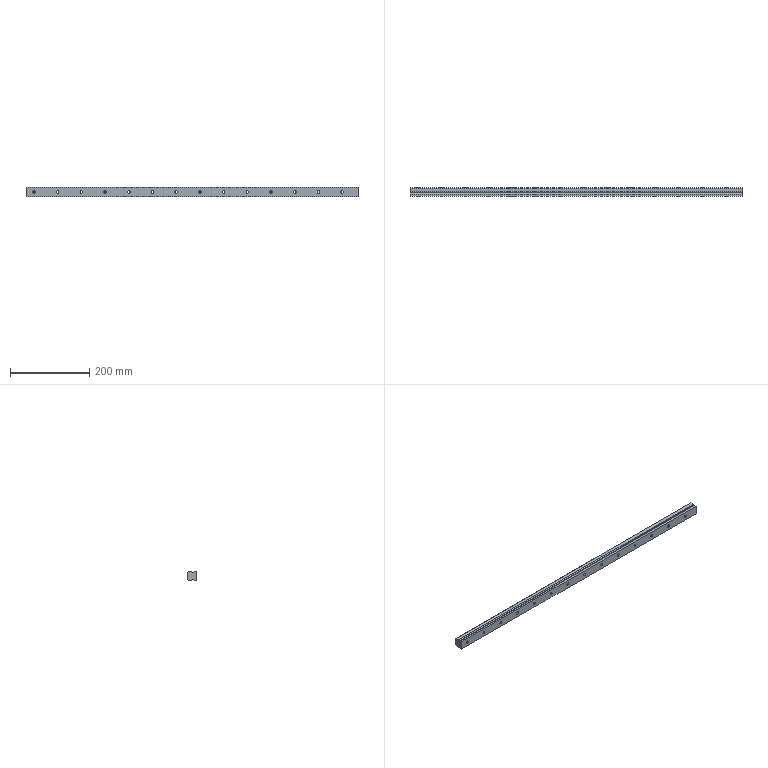Part | NX | features CBORE_HOLE 14, DATUM_CSYS 3, SKETCH 2, EXTRUDE 1, HOLE PACKAGE 1 | 1 solid | 58 faces | box 840 x 22 x 23 mm | volume 392391 mm3 | plane 30 | cylinder 28 | commonest cylinder face diameters 6.5 x14 11 x14
STEP:
#1=CARTESIAN_POINT('',(-420.,0.,-11.5));
#2=VERTEX_POINT('',#1);
#3=CARTESIAN_POINT('',(-420.,2.,-9.5));
#4=VERTEX_POINT('',#3);
#5=CARTESIAN_POINT('',(-420.,0.,-11.5));
#6=DIRECTION('',(0.,0.7071,0.7071));
#7=VECTOR('',#6,1000.);
#8=LINE('',#5,#7);
#9=EDGE_CURVE('',#2,#4,#8,.T.);
#10=ORIENTED_EDGE('',*,*,#9,.T.);
#11=CARTESIAN_POINT('',(420.,2.,-9.5));
#12=VERTEX_POINT('',#11);
#13=CARTESIAN_POINT('',(420.,2.,-9.5));
#14=DIRECTION('',(-1.,0.,0.));
#15=VECTOR('',#14,1000.);
#16=LINE('',#13,#15);
#17=EDGE_CURVE('',#12,#4,#16,.T.);
#18=ORIENTED_EDGE('',*,*,#17,.F.);
#19=CARTESIAN_POINT('',(420.,0.,-11.5));
#20=VERTEX_POINT('',#19);
#21=CARTESIAN_POINT('',(420.,0.,-11.5));
#22=DIRECTION('',(0.,0.7071,0.7071));
#23=VECTOR('',#22,1000.);
#24=LINE('',#21,#23);
#25=EDGE_CURVE('',#20,#12,#24,.T.);
#26=ORIENTED_EDGE('',*,*,#25,.F.);
#27=CARTESIAN_POINT('',(420.,0.,-11.5));
#28=DIRECTION('',(-1.,0.,0.));
#29=VECTOR('',#28,1000.);
#30=LINE('',#27,#29);
#31=EDGE_CURVE('',#20,#2,#30,.T.);
#32=ORIENTED_EDGE('',*,*,#31,.T.);
#33=EDGE_LOOP('',(#10,#18,#26,#32));
#34=FACE_BOUND('',#33,.T.);
#35=CARTESIAN_POINT('',(420.,0.,-11.5));
#36=DIRECTION('',(0.,-0.7071,0.7071));
#37=DIRECTION('',(0.,-0.7071,-0.7071));
#38=AXIS2_PLACEMENT_3D('',#35,#36,#37);
#39=PLANE('',#38);
#40=ADVANCED_FACE('',(#34),#39,.F.);
#41=CARTESIAN_POINT('',(-420.,4.,-9.5));
#42=VERTEX_POINT('',#41);
#43=CARTESIAN_POINT('',(-420.,2.,-9.5));
#44=DIRECTION('',(0.,1.,0.));
#45=VECTOR('',#44,1000.);
#46=LINE('',#43,#45);
#47=EDGE_CURVE('',#4,#42,#46,.T.);
#48=ORIENTED_EDGE('',*,*,#47,.T.);
#49=CARTESIAN_POINT('',(420.,4.,-9.5));
#50=VERTEX_POINT('',#49);
#51=CARTESIAN_POINT('',(420.,4.,-9.5));
#52=DIRECTION('',(-1.,0.,0.));
#53=VECTOR('',#52,1000.);
#54=LINE('',#51,#53);
#55=EDGE_CURVE('',#50,#42,#54,.T.);
#56=ORIENTED_EDGE('',*,*,#55,.F.);
#57=CARTESIAN_POINT('',(420.,2.,-9.5));
#58=DIRECTION('',(0.,1.,0.));
#59=VECTOR('',#58,1000.);
#60=LINE('',#57,#59);
#61=EDGE_CURVE('',#12,#50,#60,.T.);
#62=ORIENTED_EDGE('',*,*,#61,.F.);
#63=ORIENTED_EDGE('',*,*,#17,.T.);
#64=EDGE_LOOP('',(#48,#56,#62,#63));
#65=FACE_BOUND('',#64,.T.);
#66=CARTESIAN_POINT('',(420.,2.,-9.5));
#67=DIRECTION('',(0.,0.,1.));
#68=DIRECTION('',(1.,0.,0.));
#69=AXIS2_PLACEMENT_3D('',#66,#67,#68);
#70=PLANE('',#69);
#71=ADVANCED_FACE('',(#65),#70,.F.);
#72=CARTESIAN_POINT('',(-420.,6.,-11.5));
#73=VERTEX_POINT('',#72);
#74=CARTESIAN_POINT('',(-420.,4.,-9.5));
#75=DIRECTION('',(0.,0.7071,-0.7071));
#76=VECTOR('',#75,1000.);
#77=LINE('',#74,#76);
#78=EDGE_CURVE('',#42,#73,#77,.T.);
#79=ORIENTED_EDGE('',*,*,#78,.T.);
#80=CARTESIAN_POINT('',(420.,6.,-11.5));
#81=VERTEX_POINT('',#80);
#82=CARTESIAN_POINT('',(420.,6.,-11.5));
#83=DIRECTION('',(-1.,0.,0.));
#84=VECTOR('',#83,1000.);
#85=LINE('',#82,#84);
#86=EDGE_CURVE('',#81,#73,#85,.T.);
#87=ORIENTED_EDGE('',*,*,#86,.F.);
#88=CARTESIAN_POINT('',(420.,4.,-9.5));
#89=DIRECTION('',(0.,0.7071,-0.7071));
#90=VECTOR('',#89,1000.);
#91=LINE('',#88,#90);
#92=EDGE_CURVE('',#50,#81,#91,.T.);
#93=ORIENTED_EDGE('',*,*,#92,.F.);
#94=ORIENTED_EDGE('',*,*,#55,.T.);
#95=EDGE_LOOP('',(#79,#87,#93,#94));
#96=FACE_BOUND('',#95,.T.);
#97=CARTESIAN_POINT('',(420.,4.,-9.5));
#98=DIRECTION('',(0.,0.7071,0.7071));
#99=DIRECTION('',(0.,-0.7071,0.7071));
#100=AXIS2_PLACEMENT_3D('',#97,#98,#99);
#101=PLANE('',#100);
#102=ADVANCED_FACE('',(#96),#101,.F.);
#103=CARTESIAN_POINT('',(-420.,14.5,-11.5));
#104=VERTEX_POINT('',#103);
#105=CARTESIAN_POINT('',(-420.,6.,-11.5));
#106=DIRECTION('',(0.,1.,0.));
#107=VECTOR('',#106,1000.);
#108=LINE('',#105,#107);
#109=EDGE_CURVE('',#73,#104,#108,.T.);
#110=ORIENTED_EDGE('',*,*,#109,.T.);
#111=CARTESIAN_POINT('',(420.,14.5,-11.5));
#112=VERTEX_POINT('',#111);
#113=CARTESIAN_POINT('',(420.,14.5,-11.5));
#114=DIRECTION('',(-1.,0.,0.));
#115=VECTOR('',#114,1000.);
#116=LINE('',#113,#115);
#117=EDGE_CURVE('',#112,#104,#116,.T.);
#118=ORIENTED_EDGE('',*,*,#117,.F.);
#119=CARTESIAN_POINT('',(420.,6.,-11.5));
#120=DIRECTION('',(0.,1.,0.));
#121=VECTOR('',#120,1000.);
#122=LINE('',#119,#121);
#123=EDGE_CURVE('',#81,#112,#122,.T.);
#124=ORIENTED_EDGE('',*,*,#123,.F.);
#125=ORIENTED_EDGE('',*,*,#86,.T.);
#126=EDGE_LOOP('',(#110,#118,#124,#125));
#127=FACE_BOUND('',#126,.T.);
#128=CARTESIAN_POINT('',(420.,6.,-11.5));
#129=DIRECTION('',(0.,0.,1.));
#130=DIRECTION('',(0.,-1.,0.));
#131=AXIS2_PLACEMENT_3D('',#128,#129,#130);
#132=PLANE('',#131);
#133=ADVANCED_FACE('',(#127),#132,.F.);
#134=CARTESIAN_POINT('',(-420.,16.5,-9.5));
#135=VERTEX_POINT('',#134);
#136=CARTESIAN_POINT('',(-420.,14.5,-11.5));
#137=DIRECTION('',(0.,0.7071,0.7071));
#138=VECTOR('',#137,1000.);
#139=LINE('',#136,#138);
#140=EDGE_CURVE('',#104,#135,#139,.T.);
#141=ORIENTED_EDGE('',*,*,#140,.T.);
#142=CARTESIAN_POINT('',(420.,16.5,-9.5));
#143=VERTEX_POINT('',#142);
#144=CARTESIAN_POINT('',(420.,16.5,-9.5));
#145=DIRECTION('',(-1.,0.,0.));
#146=VECTOR('',#145,1000.);
#147=LINE('',#144,#146);
#148=EDGE_CURVE('',#143,#135,#147,.T.);
#149=ORIENTED_EDGE('',*,*,#148,.F.);
#150=CARTESIAN_POINT('',(420.,14.5,-11.5));
#151=DIRECTION('',(0.,0.7071,0.7071));
#152=VECTOR('',#151,1000.);
#153=LINE('',#150,#152);
#154=EDGE_CURVE('',#112,#143,#153,.T.);
#155=ORIENTED_EDGE('',*,*,#154,.F.);
#156=ORIENTED_EDGE('',*,*,#117,.T.);
#157=EDGE_LOOP('',(#141,#149,#155,#156));
#158=FACE_BOUND('',#157,.T.);
#159=CARTESIAN_POINT('',(420.,14.5,-11.5));
#160=DIRECTION('',(0.,-0.7071,0.7071));
#161=DIRECTION('',(0.,-0.7071,-0.7071));
#162=AXIS2_PLACEMENT_3D('',#159,#160,#161);
#163=PLANE('',#162);
#164=ADVANCED_FACE('',(#158),#163,.F.);
#165=CARTESIAN_POINT('',(380.,16.5,-5.5));
#166=VERTEX_POINT('',#165);
#167=CARTESIAN_POINT('',(380.,16.5,0.));
#168=DIRECTION('',(0.,-1.,0.));
#169=DIRECTION('',(0.,0.,-1.));
#170=AXIS2_PLACEMENT_3D('',#167,#168,#169);
#171=CIRCLE('',#170,5.5);
#172=EDGE_CURVE('',#166,#166,#171,.T.);
#173=ORIENTED_EDGE('',*,*,#172,.T.);
#174=EDGE_LOOP('',(#173));
#175=FACE_BOUND('',#174,.T.);
#176=CARTESIAN_POINT('',(320.,16.5,-5.5));
#177=VERTEX_POINT('',#176);
#178=CARTESIAN_POINT('',(320.,16.5,0.));
#179=DIRECTION('',(0.,-1.,0.));
#180=DIRECTION('',(0.,0.,-1.));
#181=AXIS2_PLACEMENT_3D('',#178,#179,#180);
#182=CIRCLE('',#181,5.5);
#183=EDGE_CURVE('',#177,#177,#182,.T.);
#184=ORIENTED_EDGE('',*,*,#183,.T.);
#185=EDGE_LOOP('',(#184));
#186=FACE_BOUND('',#185,.T.);
#187=CARTESIAN_POINT('',(260.,16.5,-5.5));
#188=VERTEX_POINT('',#187);
#189=CARTESIAN_POINT('',(260.,16.5,0.));
#190=DIRECTION('',(0.,-1.,0.));
#191=DIRECTION('',(0.,0.,-1.));
#192=AXIS2_PLACEMENT_3D('',#189,#190,#191);
#193=CIRCLE('',#192,5.5);
#194=EDGE_CURVE('',#188,#188,#193,.T.);
#195=ORIENTED_EDGE('',*,*,#194,.T.);
#196=EDGE_LOOP('',(#195));
#197=FACE_BOUND('',#196,.T.);
#198=CARTESIAN_POINT('',(200.,16.5,-5.5));
#199=VERTEX_POINT('',#198);
#200=CARTESIAN_POINT('',(200.,16.5,0.));
#201=DIRECTION('',(0.,-1.,0.));
#202=DIRECTION('',(0.,0.,-1.));
#203=AXIS2_PLACEMENT_3D('',#200,#201,#202);
#204=CIRCLE('',#203,5.5);
#205=EDGE_CURVE('',#199,#199,#204,.T.);
#206=ORIENTED_EDGE('',*,*,#205,.T.);
#207=EDGE_LOOP('',(#206));
#208=FACE_BOUND('',#207,.T.);
#209=CARTESIAN_POINT('',(140.,16.5,-5.5));
#210=VERTEX_POINT('',#209);
#211=CARTESIAN_POINT('',(140.,16.5,0.));
#212=DIRECTION('',(0.,-1.,0.));
#213=DIRECTION('',(0.,0.,-1.));
#214=AXIS2_PLACEMENT_3D('',#211,#212,#213);
#215=CIRCLE('',#214,5.5);
#216=EDGE_CURVE('',#210,#210,#215,.T.);
#217=ORIENTED_EDGE('',*,*,#216,.T.);
#218=EDGE_LOOP('',(#217));
#219=FACE_BOUND('',#218,.T.);
#220=CARTESIAN_POINT('',(80.,16.5,-5.5));
#221=VERTEX_POINT('',#220);
#222=CARTESIAN_POINT('',(80.,16.5,0.));
#223=DIRECTION('',(0.,-1.,0.));
#224=DIRECTION('',(0.,0.,-1.));
#225=AXIS2_PLACEMENT_3D('',#222,#223,#224);
#226=CIRCLE('',#225,5.5);
#227=EDGE_CURVE('',#221,#221,#226,.T.);
#228=ORIENTED_EDGE('',*,*,#227,.T.);
#229=EDGE_LOOP('',(#228));
#230=FACE_BOUND('',#229,.T.);
#231=CARTESIAN_POINT('',(20.,16.5,-5.5));
#232=VERTEX_POINT('',#231);
#233=CARTESIAN_POINT('',(20.,16.5,0.));
#234=DIRECTION('',(0.,-1.,0.));
#235=DIRECTION('',(0.,0.,-1.));
#236=AXIS2_PLACEMENT_3D('',#233,#234,#235);
#237=CIRCLE('',#236,5.5);
#238=EDGE_CURVE('',#232,#232,#237,.T.);
#239=ORIENTED_EDGE('',*,*,#238,.T.);
#240=EDGE_LOOP('',(#239));
#241=FACE_BOUND('',#240,.T.);
#242=CARTESIAN_POINT('',(-40.,16.5,-5.5));
#243=VERTEX_POINT('',#242);
#244=CARTESIAN_POINT('',(-40.,16.5,0.));
#245=DIRECTION('',(0.,-1.,0.));
#246=DIRECTION('',(0.,0.,-1.));
#247=AXIS2_PLACEMENT_3D('',#244,#245,#246);
#248=CIRCLE('',#247,5.5);
#249=EDGE_CURVE('',#243,#243,#248,.T.);
#250=ORIENTED_EDGE('',*,*,#249,.T.);
#251=EDGE_LOOP('',(#250));
#252=FACE_BOUND('',#251,.T.);
#253=CARTESIAN_POINT('',(-100.,16.5,-5.5));
#254=VERTEX_POINT('',#253);
#255=CARTESIAN_POINT('',(-100.,16.5,0.));
#256=DIRECTION('',(0.,-1.,0.));
#257=DIRECTION('',(0.,0.,-1.));
#258=AXIS2_PLACEMENT_3D('',#255,#256,#257);
#259=CIRCLE('',#258,5.5);
#260=EDGE_CURVE('',#254,#254,#259,.T.);
#261=ORIENTED_EDGE('',*,*,#260,.T.);
#262=EDGE_LOOP('',(#261));
#263=FACE_BOUND('',#262,.T.);
#264=CARTESIAN_POINT('',(-160.,16.5,-5.5));
#265=VERTEX_POINT('',#264);
#266=CARTESIAN_POINT('',(-160.,16.5,0.));
#267=DIRECTION('',(0.,-1.,0.));
#268=DIRECTION('',(0.,0.,-1.));
#269=AXIS2_PLACEMENT_3D('',#266,#267,#268);
#270=CIRCLE('',#269,5.5);
#271=EDGE_CURVE('',#265,#265,#270,.T.);
#272=ORIENTED_EDGE('',*,*,#271,.T.);
#273=EDGE_LOOP('',(#272));
#274=FACE_BOUND('',#273,.T.);
#275=CARTESIAN_POINT('',(-220.,16.5,-5.5));
#276=VERTEX_POINT('',#275);
#277=CARTESIAN_POINT('',(-220.,16.5,0.));
#278=DIRECTION('',(0.,-1.,0.));
#279=DIRECTION('',(0.,0.,-1.));
#280=AXIS2_PLACEMENT_3D('',#277,#278,#279);
#281=CIRCLE('',#280,5.5);
#282=EDGE_CURVE('',#276,#276,#281,.T.);
#283=ORIENTED_EDGE('',*,*,#282,.T.);
#284=EDGE_LOOP('',(#283));
#285=FACE_BOUND('',#284,.T.);
#286=CARTESIAN_POINT('',(-280.,16.5,-5.5));
#287=VERTEX_POINT('',#286);
#288=CARTESIAN_POINT('',(-280.,16.5,0.));
#289=DIRECTION('',(0.,-1.,0.));
#290=DIRECTION('',(0.,0.,-1.));
#291=AXIS2_PLACEMENT_3D('',#288,#289,#290);
#292=CIRCLE('',#291,5.5);
#293=EDGE_CURVE('',#287,#287,#292,.T.);
#294=ORIENTED_EDGE('',*,*,#293,.T.);
#295=EDGE_LOOP('',(#294));
#296=FACE_BOUND('',#295,.T.);
#297=CARTESIAN_POINT('',(-340.,16.5,-5.5));
#298=VERTEX_POINT('',#297);
#299=CARTESIAN_POINT('',(-340.,16.5,0.));
#300=DIRECTION('',(0.,-1.,0.));
#301=DIRECTION('',(0.,0.,-1.));
#302=AXIS2_PLACEMENT_3D('',#299,#300,#301);
#303=CIRCLE('',#302,5.5);
#304=EDGE_CURVE('',#298,#298,#303,.T.);
#305=ORIENTED_EDGE('',*,*,#304,.T.);
#306=EDGE_LOOP('',(#305));
#307=FACE_BOUND('',#306,.T.);
#308=CARTESIAN_POINT('',(-400.,16.5,-5.5));
#309=VERTEX_POINT('',#308);
#310=CARTESIAN_POINT('',(-400.,16.5,0.));
#311=DIRECTION('',(0.,-1.,0.));
#312=DIRECTION('',(0.,0.,-1.));
#313=AXIS2_PLACEMENT_3D('',#310,#311,#312);
#314=CIRCLE('',#313,5.5);
#315=EDGE_CURVE('',#309,#309,#314,.T.);
#316=ORIENTED_EDGE('',*,*,#315,.T.);
#317=EDGE_LOOP('',(#316));
#318=FACE_BOUND('',#317,.T.);
#319=CARTESIAN_POINT('',(-420.,16.5,9.5));
#320=VERTEX_POINT('',#319);
#321=CARTESIAN_POINT('',(-420.,16.5,0.));
#322=DIRECTION('',(0.,0.,1.));
#323=VECTOR('',#322,1000.);
#324=LINE('',#321,#323);
#325=EDGE_CURVE('',#135,#320,#324,.T.);
#326=ORIENTED_EDGE('',*,*,#325,.T.);
#327=CARTESIAN_POINT('',(420.,16.5,9.5));
#328=VERTEX_POINT('',#327);
#329=CARTESIAN_POINT('',(420.,16.5,9.5));
#330=DIRECTION('',(-1.,0.,0.));
#331=VECTOR('',#330,1000.);
#332=LINE('',#329,#331);
#333=EDGE_CURVE('',#328,#320,#332,.T.);
#334=ORIENTED_EDGE('',*,*,#333,.F.);
#335=CARTESIAN_POINT('',(420.,16.5,-9.5));
#336=DIRECTION('',(0.,0.,1.));
#337=VECTOR('',#336,1000.);
#338=LINE('',#335,#337);
#339=EDGE_CURVE('',#143,#328,#338,.T.);
#340=ORIENTED_EDGE('',*,*,#339,.F.);
#341=ORIENTED_EDGE('',*,*,#148,.T.);
#342=EDGE_LOOP('',(#326,#334,#340,#341));
#343=FACE_BOUND('',#342,.T.);
#344=CARTESIAN_POINT('',(420.,16.5,0.));
#345=DIRECTION('',(0.,-1.,0.));
#346=DIRECTION('',(0.,0.,-1.));
#347=AXIS2_PLACEMENT_3D('',#344,#345,#346);
#348=PLANE('',#347);
#349=ADVANCED_FACE('',(#175,#186,#197,#208,#219,#230,#241,#252,#263,#274,#285,#296,#307,#318,#343),#348,.F.);
#350=CARTESIAN_POINT('',(-420.,14.5,11.5));
#351=VERTEX_POINT('',#350);
#352=CARTESIAN_POINT('',(-420.,16.5,9.5));
#353=DIRECTION('',(0.,-0.7071,0.7071));
#354=VECTOR('',#353,1000.);
#355=LINE('',#352,#354);
#356=EDGE_CURVE('',#320,#351,#355,.T.);
#357=ORIENTED_EDGE('',*,*,#356,.T.);
#358=CARTESIAN_POINT('',(420.,14.5,11.5));
#359=VERTEX_POINT('',#358);
#360=CARTESIAN_POINT('',(420.,14.5,11.5));
#361=DIRECTION('',(-1.,0.,0.));
#362=VECTOR('',#361,1000.);
#363=LINE('',#360,#362);
#364=EDGE_CURVE('',#359,#351,#363,.T.);
#365=ORIENTED_EDGE('',*,*,#364,.F.);
#366=CARTESIAN_POINT('',(420.,16.5,9.5));
#367=DIRECTION('',(0.,-0.7071,0.7071));
#368=VECTOR('',#367,1000.);
#369=LINE('',#366,#368);
#370=EDGE_CURVE('',#328,#359,#369,.T.);
#371=ORIENTED_EDGE('',*,*,#370,.F.);
#372=ORIENTED_EDGE('',*,*,#333,.T.);
#373=EDGE_LOOP('',(#357,#365,#371,#372));
#374=FACE_BOUND('',#373,.T.);
#375=CARTESIAN_POINT('',(420.,16.5,9.5));
#376=DIRECTION('',(0.,-0.7071,-0.7071));
#377=DIRECTION('',(0.,0.7071,-0.7071));
#378=AXIS2_PLACEMENT_3D('',#375,#376,#377);
#379=PLANE('',#378);
#380=ADVANCED_FACE('',(#374),#379,.F.);
#381=CARTESIAN_POINT('',(-420.,6.,11.5));
#382=VERTEX_POINT('',#381);
#383=CARTESIAN_POINT('',(-420.,14.5,11.5));
#384=DIRECTION('',(0.,-1.,0.));
#385=VECTOR('',#384,1000.);
#386=LINE('',#383,#385);
#387=EDGE_CURVE('',#351,#382,#386,.T.);
#388=ORIENTED_EDGE('',*,*,#387,.T.);
#389=CARTESIAN_POINT('',(420.,6.,11.5));
#390=VERTEX_POINT('',#389);
#391=CARTESIAN_POINT('',(420.,6.,11.5));
#392=DIRECTION('',(-1.,0.,0.));
#393=VECTOR('',#392,1000.);
#394=LINE('',#391,#393);
#395=EDGE_CURVE('',#390,#382,#394,.T.);
#396=ORIENTED_EDGE('',*,*,#395,.F.);
#397=CARTESIAN_POINT('',(420.,14.5,11.5));
#398=DIRECTION('',(0.,-1.,0.));
#399=VECTOR('',#398,1000.);
#400=LINE('',#397,#399);
#401=EDGE_CURVE('',#359,#390,#400,.T.);
#402=ORIENTED_EDGE('',*,*,#401,.F.);
#403=ORIENTED_EDGE('',*,*,#364,.T.);
#404=EDGE_LOOP('',(#388,#396,#402,#403));
#405=FACE_BOUND('',#404,.T.);
#406=CARTESIAN_POINT('',(420.,14.5,11.5));
#407=DIRECTION('',(0.,0.,-1.));
#408=DIRECTION('',(0.,1.,0.));
#409=AXIS2_PLACEMENT_3D('',#406,#407,#408);
#410=PLANE('',#409);
#411=ADVANCED_FACE('',(#405),#410,.F.);
#412=CARTESIAN_POINT('',(-420.,4.,9.5));
#413=VERTEX_POINT('',#412);
#414=CARTESIAN_POINT('',(-420.,6.,11.5));
#415=DIRECTION('',(0.,-0.7071,-0.7071));
#416=VECTOR('',#415,1000.);
#417=LINE('',#414,#416);
#418=EDGE_CURVE('',#382,#413,#417,.T.);
#419=ORIENTED_EDGE('',*,*,#418,.T.);
#420=CARTESIAN_POINT('',(420.,4.,9.5));
#421=VERTEX_POINT('',#420);
#422=CARTESIAN_POINT('',(420.,4.,9.5));
#423=DIRECTION('',(-1.,0.,0.));
#424=VECTOR('',#423,1000.);
#425=LINE('',#422,#424);
#426=EDGE_CURVE('',#421,#413,#425,.T.);
#427=ORIENTED_EDGE('',*,*,#426,.F.);
#428=CARTESIAN_POINT('',(420.,6.,11.5));
#429=DIRECTION('',(0.,-0.7071,-0.7071));
#430=VECTOR('',#429,1000.);
#431=LINE('',#428,#430);
#432=EDGE_CURVE('',#390,#421,#431,.T.);
#433=ORIENTED_EDGE('',*,*,#432,.F.);
#434=ORIENTED_EDGE('',*,*,#395,.T.);
#435=EDGE_LOOP('',(#419,#427,#433,#434));
#436=FACE_BOUND('',#435,.T.);
#437=CARTESIAN_POINT('',(420.,6.,11.5));
#438=DIRECTION('',(0.,0.7071,-0.7071));
#439=DIRECTION('',(0.,0.7071,0.7071));
#440=AXIS2_PLACEMENT_3D('',#437,#438,#439);
#441=PLANE('',#440);
#442=ADVANCED_FACE('',(#436),#441,.F.);
#443=CARTESIAN_POINT('',(-420.,2.,9.5));
#444=VERTEX_POINT('',#443);
#445=CARTESIAN_POINT('',(-420.,4.,9.5));
#446=DIRECTION('',(0.,-1.,0.));
#447=VECTOR('',#446,1000.);
#448=LINE('',#445,#447);
#449=EDGE_CURVE('',#413,#444,#448,.T.);
#450=ORIENTED_EDGE('',*,*,#449,.T.);
#451=CARTESIAN_POINT('',(420.,2.,9.5));
#452=VERTEX_POINT('',#451);
#453=CARTESIAN_POINT('',(420.,2.,9.5));
#454=DIRECTION('',(-1.,0.,0.));
#455=VECTOR('',#454,1000.);
#456=LINE('',#453,#455);
#457=EDGE_CURVE('',#452,#444,#456,.T.);
#458=ORIENTED_EDGE('',*,*,#457,.F.);
#459=CARTESIAN_POINT('',(420.,4.,9.5));
#460=DIRECTION('',(0.,-1.,0.));
#461=VECTOR('',#460,1000.);
#462=LINE('',#459,#461);
#463=EDGE_CURVE('',#421,#452,#462,.T.);
#464=ORIENTED_EDGE('',*,*,#463,.F.);
#465=ORIENTED_EDGE('',*,*,#426,.T.);
#466=EDGE_LOOP('',(#450,#458,#464,#465));
#467=FACE_BOUND('',#466,.T.);
#468=CARTESIAN_POINT('',(420.,4.,9.5));
#469=DIRECTION('',(0.,0.,-1.));
#470=DIRECTION('',(-1.,0.,0.));
#471=AXIS2_PLACEMENT_3D('',#468,#469,#470);
#472=PLANE('',#471);
#473=ADVANCED_FACE('',(#467),#472,.F.);
#474=CARTESIAN_POINT('',(-420.,0.,11.5));
#475=VERTEX_POINT('',#474);
#476=CARTESIAN_POINT('',(-420.,2.,9.5));
#477=DIRECTION('',(0.,-0.7071,0.7071));
#478=VECTOR('',#477,1000.);
#479=LINE('',#476,#478);
#480=EDGE_CURVE('',#444,#475,#479,.T.);
#481=ORIENTED_EDGE('',*,*,#480,.T.);
#482=CARTESIAN_POINT('',(420.,0.,11.5));
#483=VERTEX_POINT('',#482);
#484=CARTESIAN_POINT('',(420.,0.,11.5));
#485=DIRECTION('',(-1.,0.,0.));
#486=VECTOR('',#485,1000.);
#487=LINE('',#484,#486);
#488=EDGE_CURVE('',#483,#475,#487,.T.);
#489=ORIENTED_EDGE('',*,*,#488,.F.);
#490=CARTESIAN_POINT('',(420.,2.,9.5));
#491=DIRECTION('',(0.,-0.7071,0.7071));
#492=VECTOR('',#491,1000.);
#493=LINE('',#490,#492);
#494=EDGE_CURVE('',#452,#483,#493,.T.);
#495=ORIENTED_EDGE('',*,*,#494,.F.);
#496=ORIENTED_EDGE('',*,*,#457,.T.);
#497=EDGE_LOOP('',(#481,#489,#495,#496));
#498=FACE_BOUND('',#497,.T.);
#499=CARTESIAN_POINT('',(420.,2.,9.5));
#500=DIRECTION('',(0.,-0.7071,-0.7071));
#501=DIRECTION('',(0.,0.7071,-0.7071));
#502=AXIS2_PLACEMENT_3D('',#499,#500,#501);
#503=PLANE('',#502);
#504=ADVANCED_FACE('',(#498),#503,.F.);
#505=CARTESIAN_POINT('',(-420.,-5.5,11.5));
#506=VERTEX_POINT('',#505);
#507=CARTESIAN_POINT('',(-420.,0.,11.5));
#508=DIRECTION('',(0.,-1.,0.));
#509=VECTOR('',#508,1000.);
#510=LINE('',#507,#509);
#511=EDGE_CURVE('',#475,#506,#510,.T.);
#512=ORIENTED_EDGE('',*,*,#511,.T.);
#513=CARTESIAN_POINT('',(420.,-5.5,11.5));
#514=VERTEX_POINT('',#513);
#515=CARTESIAN_POINT('',(420.,-5.5,11.5));
#516=DIRECTION('',(-1.,0.,0.));
#517=VECTOR('',#516,1000.);
#518=LINE('',#515,#517);
#519=EDGE_CURVE('',#514,#506,#518,.T.);
#520=ORIENTED_EDGE('',*,*,#519,.F.);
#521=CARTESIAN_POINT('',(420.,0.,11.5));
#522=DIRECTION('',(0.,-1.,0.));
#523=VECTOR('',#522,1000.);
#524=LINE('',#521,#523);
#525=EDGE_CURVE('',#483,#514,#524,.T.);
#526=ORIENTED_EDGE('',*,*,#525,.F.);
#527=ORIENTED_EDGE('',*,*,#488,.T.);
#528=EDGE_LOOP('',(#512,#520,#526,#527));
#529=FACE_BOUND('',#528,.T.);
#530=CARTESIAN_POINT('',(420.,0.,11.5));
#531=DIRECTION('',(0.,0.,-1.));
#532=DIRECTION('',(0.,1.,0.));
#533=AXIS2_PLACEMENT_3D('',#530,#531,#532);
#534=PLANE('',#533);
#535=ADVANCED_FACE('',(#529),#534,.F.);
#536=CARTESIAN_POINT('',(380.,-5.5,3.25));
#537=VERTEX_POINT('',#536);
#538=CARTESIAN_POINT('',(380.,-5.5,0.));
#539=DIRECTION('',(0.,1.,0.));
#540=DIRECTION('',(0.,0.,1.));
#541=AXIS2_PLACEMENT_3D('',#538,#539,#540);
#542=CIRCLE('',#541,3.25);
#543=EDGE_CURVE('',#537,#537,#542,.T.);
#544=ORIENTED_EDGE('',*,*,#543,.T.);
#545=EDGE_LOOP('',(#544));
#546=FACE_BOUND('',#545,.T.);
#547=CARTESIAN_POINT('',(320.,-5.5,3.25));
#548=VERTEX_POINT('',#547);
#549=CARTESIAN_POINT('',(320.,-5.5,0.));
#550=DIRECTION('',(0.,1.,0.));
#551=DIRECTION('',(0.,0.,1.));
#552=AXIS2_PLACEMENT_3D('',#549,#550,#551);
#553=CIRCLE('',#552,3.25);
#554=EDGE_CURVE('',#548,#548,#553,.T.);
#555=ORIENTED_EDGE('',*,*,#554,.T.);
#556=EDGE_LOOP('',(#555));
#557=FACE_BOUND('',#556,.T.);
#558=CARTESIAN_POINT('',(260.,-5.5,3.25));
#559=VERTEX_POINT('',#558);
#560=CARTESIAN_POINT('',(260.,-5.5,0.));
#561=DIRECTION('',(0.,1.,0.));
#562=DIRECTION('',(0.,0.,1.));
#563=AXIS2_PLACEMENT_3D('',#560,#561,#562);
#564=CIRCLE('',#563,3.25);
#565=EDGE_CURVE('',#559,#559,#564,.T.);
#566=ORIENTED_EDGE('',*,*,#565,.T.);
#567=EDGE_LOOP('',(#566));
#568=FACE_BOUND('',#567,.T.);
#569=CARTESIAN_POINT('',(200.,-5.5,3.25));
#570=VERTEX_POINT('',#569);
#571=CARTESIAN_POINT('',(200.,-5.5,0.));
#572=DIRECTION('',(0.,1.,0.));
#573=DIRECTION('',(0.,0.,1.));
#574=AXIS2_PLACEMENT_3D('',#571,#572,#573);
#575=CIRCLE('',#574,3.25);
#576=EDGE_CURVE('',#570,#570,#575,.T.);
#577=ORIENTED_EDGE('',*,*,#576,.T.);
#578=EDGE_LOOP('',(#577));
#579=FACE_BOUND('',#578,.T.);
#580=CARTESIAN_POINT('',(140.,-5.5,3.25));
#581=VERTEX_POINT('',#580);
#582=CARTESIAN_POINT('',(140.,-5.5,0.));
#583=DIRECTION('',(0.,1.,0.));
#584=DIRECTION('',(0.,0.,1.));
#585=AXIS2_PLACEMENT_3D('',#582,#583,#584);
#586=CIRCLE('',#585,3.25);
#587=EDGE_CURVE('',#581,#581,#586,.T.);
#588=ORIENTED_EDGE('',*,*,#587,.T.);
#589=EDGE_LOOP('',(#588));
#590=FACE_BOUND('',#589,.T.);
#591=CARTESIAN_POINT('',(80.,-5.5,3.25));
#592=VERTEX_POINT('',#591);
#593=CARTESIAN_POINT('',(80.,-5.5,0.));
#594=DIRECTION('',(0.,1.,0.));
#595=DIRECTION('',(0.,0.,1.));
#596=AXIS2_PLACEMENT_3D('',#593,#594,#595);
#597=CIRCLE('',#596,3.25);
#598=EDGE_CURVE('',#592,#592,#597,.T.);
#599=ORIENTED_EDGE('',*,*,#598,.T.);
#600=EDGE_LOOP('',(#599));
#601=FACE_BOUND('',#600,.T.);
#602=CARTESIAN_POINT('',(20.,-5.5,3.25));
#603=VERTEX_POINT('',#602);
#604=CARTESIAN_POINT('',(20.,-5.5,0.));
#605=DIRECTION('',(0.,1.,0.));
#606=DIRECTION('',(0.,0.,1.));
#607=AXIS2_PLACEMENT_3D('',#604,#605,#606);
#608=CIRCLE('',#607,3.25);
#609=EDGE_CURVE('',#603,#603,#608,.T.);
#610=ORIENTED_EDGE('',*,*,#609,.T.);
#611=EDGE_LOOP('',(#610));
#612=FACE_BOUND('',#611,.T.);
#613=CARTESIAN_POINT('',(-40.,-5.5,3.25));
#614=VERTEX_POINT('',#613);
#615=CARTESIAN_POINT('',(-40.,-5.5,0.));
#616=DIRECTION('',(0.,1.,0.));
#617=DIRECTION('',(0.,0.,1.));
#618=AXIS2_PLACEMENT_3D('',#615,#616,#617);
#619=CIRCLE('',#618,3.25);
#620=EDGE_CURVE('',#614,#614,#619,.T.);
#621=ORIENTED_EDGE('',*,*,#620,.T.);
#622=EDGE_LOOP('',(#621));
#623=FACE_BOUND('',#622,.T.);
#624=CARTESIAN_POINT('',(-100.,-5.5,3.25));
#625=VERTEX_POINT('',#624);
#626=CARTESIAN_POINT('',(-100.,-5.5,0.));
#627=DIRECTION('',(0.,1.,0.));
#628=DIRECTION('',(0.,0.,1.));
#629=AXIS2_PLACEMENT_3D('',#626,#627,#628);
#630=CIRCLE('',#629,3.25);
#631=EDGE_CURVE('',#625,#625,#630,.T.);
#632=ORIENTED_EDGE('',*,*,#631,.T.);
#633=EDGE_LOOP('',(#632));
#634=FACE_BOUND('',#633,.T.);
#635=CARTESIAN_POINT('',(-160.,-5.5,3.25));
#636=VERTEX_POINT('',#635);
#637=CARTESIAN_POINT('',(-160.,-5.5,0.));
#638=DIRECTION('',(0.,1.,0.));
#639=DIRECTION('',(0.,0.,1.));
#640=AXIS2_PLACEMENT_3D('',#637,#638,#639);
#641=CIRCLE('',#640,3.25);
#642=EDGE_CURVE('',#636,#636,#641,.T.);
#643=ORIENTED_EDGE('',*,*,#642,.T.);
#644=EDGE_LOOP('',(#643));
#645=FACE_BOUND('',#644,.T.);
#646=CARTESIAN_POINT('',(-220.,-5.5,3.25));
#647=VERTEX_POINT('',#646);
#648=CARTESIAN_POINT('',(-220.,-5.5,0.));
#649=DIRECTION('',(0.,1.,0.));
#650=DIRECTION('',(0.,0.,1.));
#651=AXIS2_PLACEMENT_3D('',#648,#649,#650);
#652=CIRCLE('',#651,3.25);
#653=EDGE_CURVE('',#647,#647,#652,.T.);
#654=ORIENTED_EDGE('',*,*,#653,.T.);
#655=EDGE_LOOP('',(#654));
#656=FACE_BOUND('',#655,.T.);
#657=CARTESIAN_POINT('',(-280.,-5.5,3.25));
#658=VERTEX_POINT('',#657);
#659=CARTESIAN_POINT('',(-280.,-5.5,0.));
#660=DIRECTION('',(0.,1.,0.));
#661=DIRECTION('',(0.,0.,1.));
#662=AXIS2_PLACEMENT_3D('',#659,#660,#661);
#663=CIRCLE('',#662,3.25);
#664=EDGE_CURVE('',#658,#658,#663,.T.);
#665=ORIENTED_EDGE('',*,*,#664,.T.);
#666=EDGE_LOOP('',(#665));
#667=FACE_BOUND('',#666,.T.);
#668=CARTESIAN_POINT('',(-340.,-5.5,3.25));
#669=VERTEX_POINT('',#668);
#670=CARTESIAN_POINT('',(-340.,-5.5,0.));
#671=DIRECTION('',(0.,1.,0.));
#672=DIRECTION('',(0.,0.,1.));
#673=AXIS2_PLACEMENT_3D('',#670,#671,#672);
#674=CIRCLE('',#673,3.25);
#675=EDGE_CURVE('',#669,#669,#674,.T.);
#676=ORIENTED_EDGE('',*,*,#675,.T.);
#677=EDGE_LOOP('',(#676));
#678=FACE_BOUND('',#677,.T.);
#679=CARTESIAN_POINT('',(-400.,-5.5,3.25));
#680=VERTEX_POINT('',#679);
#681=CARTESIAN_POINT('',(-400.,-5.5,0.));
#682=DIRECTION('',(0.,1.,0.));
#683=DIRECTION('',(0.,0.,1.));
#684=AXIS2_PLACEMENT_3D('',#681,#682,#683);
#685=CIRCLE('',#684,3.25);
#686=EDGE_CURVE('',#680,#680,#685,.T.);
#687=ORIENTED_EDGE('',*,*,#686,.T.);
#688=EDGE_LOOP('',(#687));
#689=FACE_BOUND('',#688,.T.);
#690=CARTESIAN_POINT('',(-420.,-5.5,-11.5));
#691=VERTEX_POINT('',#690);
#692=CARTESIAN_POINT('',(-420.,-5.5,11.5));
#693=DIRECTION('',(0.,0.,-1.));
#694=VECTOR('',#693,1000.);
#695=LINE('',#692,#694);
#696=EDGE_CURVE('',#506,#691,#695,.T.);
#697=ORIENTED_EDGE('',*,*,#696,.T.);
#698=CARTESIAN_POINT('',(420.,-5.5,-11.5));
#699=VERTEX_POINT('',#698);
#700=CARTESIAN_POINT('',(420.,-5.5,-11.5));
#701=DIRECTION('',(-1.,0.,0.));
#702=VECTOR('',#701,1000.);
#703=LINE('',#700,#702);
#704=EDGE_CURVE('',#699,#691,#703,.T.);
#705=ORIENTED_EDGE('',*,*,#704,.F.);
#706=CARTESIAN_POINT('',(420.,-5.5,11.5));
#707=DIRECTION('',(0.,0.,-1.));
#708=VECTOR('',#707,1000.);
#709=LINE('',#706,#708);
#710=EDGE_CURVE('',#514,#699,#709,.T.);
#711=ORIENTED_EDGE('',*,*,#710,.F.);
#712=ORIENTED_EDGE('',*,*,#519,.T.);
#713=EDGE_LOOP('',(#697,#705,#711,#712));
#714=FACE_BOUND('',#713,.T.);
#715=CARTESIAN_POINT('',(420.,-5.5,11.5));
#716=DIRECTION('',(0.,1.,0.));
#717=DIRECTION('',(0.,0.,1.));
#718=AXIS2_PLACEMENT_3D('',#715,#716,#717);
#719=PLANE('',#718);
#720=ADVANCED_FACE('',(#546,#557,#568,#579,#590,#601,#612,#623,#634,#645,#656,#667,#678,#689,#714),#719,.F.);
#721=CARTESIAN_POINT('',(-420.,-5.5,-11.5));
#722=DIRECTION('',(0.,1.,0.));
#723=VECTOR('',#722,1000.);
#724=LINE('',#721,#723);
#725=EDGE_CURVE('',#691,#2,#724,.T.);
#726=ORIENTED_EDGE('',*,*,#725,.T.);
#727=ORIENTED_EDGE('',*,*,#31,.F.);
#728=CARTESIAN_POINT('',(420.,-5.5,-11.5));
#729=DIRECTION('',(0.,1.,0.));
#730=VECTOR('',#729,1000.);
#731=LINE('',#728,#730);
#732=EDGE_CURVE('',#699,#20,#731,.T.);
#733=ORIENTED_EDGE('',*,*,#732,.F.);
#734=ORIENTED_EDGE('',*,*,#704,.T.);
#735=EDGE_LOOP('',(#726,#727,#733,#734));
#736=FACE_BOUND('',#735,.T.);
#737=CARTESIAN_POINT('',(420.,-5.5,-11.5));
#738=DIRECTION('',(0.,0.,1.));
#739=DIRECTION('',(0.,-1.,0.));
#740=AXIS2_PLACEMENT_3D('',#737,#738,#739);
#741=PLANE('',#740);
#742=ADVANCED_FACE('',(#736),#741,.F.);
#743=ORIENTED_EDGE('',*,*,#25,.T.);
#744=ORIENTED_EDGE('',*,*,#61,.T.);
#745=ORIENTED_EDGE('',*,*,#92,.T.);
#746=ORIENTED_EDGE('',*,*,#123,.T.);
#747=ORIENTED_EDGE('',*,*,#154,.T.);
#748=ORIENTED_EDGE('',*,*,#339,.T.);
#749=ORIENTED_EDGE('',*,*,#370,.T.);
#750=ORIENTED_EDGE('',*,*,#401,.T.);
#751=ORIENTED_EDGE('',*,*,#432,.T.);
#752=ORIENTED_EDGE('',*,*,#463,.T.);
#753=ORIENTED_EDGE('',*,*,#494,.T.);
#754=ORIENTED_EDGE('',*,*,#525,.T.);
#755=ORIENTED_EDGE('',*,*,#710,.T.);
#756=ORIENTED_EDGE('',*,*,#732,.T.);
#757=EDGE_LOOP('',(#743,#744,#745,#746,#747,#748,#749,#750,#751,#752,#753,#754,#755,#756));
#758=FACE_BOUND('',#757,.T.);
#759=CARTESIAN_POINT('',(420.,0.,0.));
#760=DIRECTION('',(-1.,0.,0.));
#761=DIRECTION('',(0.,0.,1.));
#762=AXIS2_PLACEMENT_3D('',#759,#760,#761);
#763=PLANE('',#762);
#764=ADVANCED_FACE('',(#758),#763,.F.);
#765=ORIENTED_EDGE('',*,*,#9,.F.);
#766=ORIENTED_EDGE('',*,*,#725,.F.);
#767=ORIENTED_EDGE('',*,*,#696,.F.);
#768=ORIENTED_EDGE('',*,*,#511,.F.);
#769=ORIENTED_EDGE('',*,*,#480,.F.);
#770=ORIENTED_EDGE('',*,*,#449,.F.);
#771=ORIENTED_EDGE('',*,*,#418,.F.);
#772=ORIENTED_EDGE('',*,*,#387,.F.);
#773=ORIENTED_EDGE('',*,*,#356,.F.);
#774=ORIENTED_EDGE('',*,*,#325,.F.);
#775=ORIENTED_EDGE('',*,*,#140,.F.);
#776=ORIENTED_EDGE('',*,*,#109,.F.);
#777=ORIENTED_EDGE('',*,*,#78,.F.);
#778=ORIENTED_EDGE('',*,*,#47,.F.);
#779=EDGE_LOOP('',(#765,#766,#767,#768,#769,#770,#771,#772,#773,#774,#775,#776,#777,#778));
#780=FACE_BOUND('',#779,.T.);
#781=CARTESIAN_POINT('',(-420.,0.,0.));
#782=DIRECTION('',(-1.,0.,0.));
#783=DIRECTION('',(0.,0.,1.));
#784=AXIS2_PLACEMENT_3D('',#781,#782,#783);
#785=PLANE('',#784);
#786=ADVANCED_FACE('',(#780),#785,.T.);
#787=CARTESIAN_POINT('',(-400.,10.,-3.25));
#788=VERTEX_POINT('',#787);
#789=CARTESIAN_POINT('',(-400.,10.,0.));
#790=DIRECTION('',(0.,-1.,0.));
#791=DIRECTION('',(0.,0.,-1.));
#792=AXIS2_PLACEMENT_3D('',#789,#790,#791);
#793=CIRCLE('',#792,3.25);
#794=EDGE_CURVE('',#788,#788,#793,.F.);
#795=ORIENTED_EDGE('',*,*,#794,.T.);
#796=EDGE_LOOP('',(#795));
#797=FACE_BOUND('',#796,.T.);
#798=ORIENTED_EDGE('',*,*,#686,.F.);
#799=EDGE_LOOP('',(#798));
#800=FACE_BOUND('',#799,.T.);
#801=CARTESIAN_POINT('',(-400.,-226.341,0.));
#802=DIRECTION('',(0.,-1.,0.));
#803=DIRECTION('',(0.,0.,-1.));
#804=AXIS2_PLACEMENT_3D('',#801,#802,#803);
#805=CYLINDRICAL_SURFACE('',#804,3.25);
#806=ADVANCED_FACE('',(#797,#800),#805,.F.);
#807=ORIENTED_EDGE('',*,*,#794,.F.);
#808=EDGE_LOOP('',(#807));
#809=FACE_BOUND('',#808,.T.);
#810=CARTESIAN_POINT('',(-400.,10.,-5.5));
#811=VERTEX_POINT('',#810);
#812=CARTESIAN_POINT('',(-400.,10.,0.));
#813=DIRECTION('',(0.,-1.,0.));
#814=DIRECTION('',(0.,0.,-1.));
#815=AXIS2_PLACEMENT_3D('',#812,#813,#814);
#816=CIRCLE('',#815,5.5);
#817=EDGE_CURVE('',#811,#811,#816,.F.);
#818=ORIENTED_EDGE('',*,*,#817,.T.);
#819=EDGE_LOOP('',(#818));
#820=FACE_BOUND('',#819,.T.);
#821=CARTESIAN_POINT('',(-400.,10.,0.));
#822=DIRECTION('',(0.,-1.,0.));
#823=DIRECTION('',(0.,0.,-1.));
#824=AXIS2_PLACEMENT_3D('',#821,#822,#823);
#825=PLANE('',#824);
#826=ADVANCED_FACE('',(#809,#820),#825,.F.);
#827=ORIENTED_EDGE('',*,*,#817,.F.);
#828=EDGE_LOOP('',(#827));
#829=FACE_BOUND('',#828,.T.);
#830=ORIENTED_EDGE('',*,*,#315,.F.);
#831=EDGE_LOOP('',(#830));
#832=FACE_BOUND('',#831,.T.);
#833=CARTESIAN_POINT('',(-400.,16.5,0.));
#834=DIRECTION('',(0.,-1.,0.));
#835=DIRECTION('',(0.,0.,-1.));
#836=AXIS2_PLACEMENT_3D('',#833,#834,#835);
#837=CYLINDRICAL_SURFACE('',#836,5.5);
#838=ADVANCED_FACE('',(#829,#832),#837,.F.);
#839=CARTESIAN_POINT('',(-340.,10.,-3.25));
#840=VERTEX_POINT('',#839);
#841=CARTESIAN_POINT('',(-340.,10.,0.));
#842=DIRECTION('',(0.,-1.,0.));
#843=DIRECTION('',(0.,0.,-1.));
#844=AXIS2_PLACEMENT_3D('',#841,#842,#843);
#845=CIRCLE('',#844,3.25);
#846=EDGE_CURVE('',#840,#840,#845,.F.);
#847=ORIENTED_EDGE('',*,*,#846,.T.);
#848=EDGE_LOOP('',(#847));
#849=FACE_BOUND('',#848,.T.);
#850=ORIENTED_EDGE('',*,*,#675,.F.);
#851=EDGE_LOOP('',(#850));
#852=FACE_BOUND('',#851,.T.);
#853=CARTESIAN_POINT('',(-340.,-307.79,0.));
#854=DIRECTION('',(0.,-1.,0.));
#855=DIRECTION('',(0.,0.,-1.));
#856=AXIS2_PLACEMENT_3D('',#853,#854,#855);
#857=CYLINDRICAL_SURFACE('',#856,3.25);
#858=ADVANCED_FACE('',(#849,#852),#857,.F.);
#859=ORIENTED_EDGE('',*,*,#846,.F.);
#860=EDGE_LOOP('',(#859));
#861=FACE_BOUND('',#860,.T.);
#862=CARTESIAN_POINT('',(-340.,10.,-5.5));
#863=VERTEX_POINT('',#862);
#864=CARTESIAN_POINT('',(-340.,10.,0.));
#865=DIRECTION('',(0.,-1.,0.));
#866=DIRECTION('',(0.,0.,-1.));
#867=AXIS2_PLACEMENT_3D('',#864,#865,#866);
#868=CIRCLE('',#867,5.5);
#869=EDGE_CURVE('',#863,#863,#868,.F.);
#870=ORIENTED_EDGE('',*,*,#869,.T.);
#871=EDGE_LOOP('',(#870));
#872=FACE_BOUND('',#871,.T.);
#873=CARTESIAN_POINT('',(-340.,10.,0.));
#874=DIRECTION('',(0.,-1.,0.));
#875=DIRECTION('',(0.,0.,-1.));
#876=AXIS2_PLACEMENT_3D('',#873,#874,#875);
#877=PLANE('',#876);
#878=ADVANCED_FACE('',(#861,#872),#877,.F.);
#879=ORIENTED_EDGE('',*,*,#869,.F.);
#880=EDGE_LOOP('',(#879));
#881=FACE_BOUND('',#880,.T.);
#882=ORIENTED_EDGE('',*,*,#304,.F.);
#883=EDGE_LOOP('',(#882));
#884=FACE_BOUND('',#883,.T.);
#885=CARTESIAN_POINT('',(-340.,16.5,0.));
#886=DIRECTION('',(0.,-1.,0.));
#887=DIRECTION('',(0.,0.,-1.));
#888=AXIS2_PLACEMENT_3D('',#885,#886,#887);
#889=CYLINDRICAL_SURFACE('',#888,5.5);
#890=ADVANCED_FACE('',(#881,#884),#889,.F.);
#891=CARTESIAN_POINT('',(-280.,10.,-3.25));
#892=VERTEX_POINT('',#891);
#893=CARTESIAN_POINT('',(-280.,10.,0.));
#894=DIRECTION('',(0.,-1.,0.));
#895=DIRECTION('',(0.,0.,-1.));
#896=AXIS2_PLACEMENT_3D('',#893,#894,#895);
#897=CIRCLE('',#896,3.25);
#898=EDGE_CURVE('',#892,#892,#897,.F.);
#899=ORIENTED_EDGE('',*,*,#898,.T.);
#900=EDGE_LOOP('',(#899));
#901=FACE_BOUND('',#900,.T.);
#902=ORIENTED_EDGE('',*,*,#664,.F.);
#903=EDGE_LOOP('',(#902));
#904=FACE_BOUND('',#903,.T.);
#905=CARTESIAN_POINT('',(-280.,-362.4,0.));
#906=DIRECTION('',(0.,-1.,0.));
#907=DIRECTION('',(0.,0.,-1.));
#908=AXIS2_PLACEMENT_3D('',#905,#906,#907);
#909=CYLINDRICAL_SURFACE('',#908,3.25);
#910=ADVANCED_FACE('',(#901,#904),#909,.F.);
#911=ORIENTED_EDGE('',*,*,#898,.F.);
#912=EDGE_LOOP('',(#911));
#913=FACE_BOUND('',#912,.T.);
#914=CARTESIAN_POINT('',(-280.,10.,-5.5));
#915=VERTEX_POINT('',#914);
#916=CARTESIAN_POINT('',(-280.,10.,0.));
#917=DIRECTION('',(0.,-1.,0.));
#918=DIRECTION('',(0.,0.,-1.));
#919=AXIS2_PLACEMENT_3D('',#916,#917,#918);
#920=CIRCLE('',#919,5.5);
#921=EDGE_CURVE('',#915,#915,#920,.F.);
#922=ORIENTED_EDGE('',*,*,#921,.T.);
#923=EDGE_LOOP('',(#922));
#924=FACE_BOUND('',#923,.T.);
#925=CARTESIAN_POINT('',(-280.,10.,0.));
#926=DIRECTION('',(0.,-1.,0.));
#927=DIRECTION('',(0.,0.,-1.));
#928=AXIS2_PLACEMENT_3D('',#925,#926,#927);
#929=PLANE('',#928);
#930=ADVANCED_FACE('',(#913,#924),#929,.F.);
#931=ORIENTED_EDGE('',*,*,#921,.F.);
#932=EDGE_LOOP('',(#931));
#933=FACE_BOUND('',#932,.T.);
#934=ORIENTED_EDGE('',*,*,#293,.F.);
#935=EDGE_LOOP('',(#934));
#936=FACE_BOUND('',#935,.T.);
#937=CARTESIAN_POINT('',(-280.,16.5,0.));
#938=DIRECTION('',(0.,-1.,0.));
#939=DIRECTION('',(0.,0.,-1.));
#940=AXIS2_PLACEMENT_3D('',#937,#938,#939);
#941=CYLINDRICAL_SURFACE('',#940,5.5);
#942=ADVANCED_FACE('',(#933,#936),#941,.F.);
#943=CARTESIAN_POINT('',(-220.,10.,-3.25));
#944=VERTEX_POINT('',#943);
#945=CARTESIAN_POINT('',(-220.,10.,0.));
#946=DIRECTION('',(0.,-1.,0.));
#947=DIRECTION('',(0.,0.,-1.));
#948=AXIS2_PLACEMENT_3D('',#945,#946,#947);
#949=CIRCLE('',#948,3.25);
#950=EDGE_CURVE('',#944,#944,#949,.F.);
#951=ORIENTED_EDGE('',*,*,#950,.T.);
#952=EDGE_LOOP('',(#951));
#953=FACE_BOUND('',#952,.T.);
#954=ORIENTED_EDGE('',*,*,#653,.F.);
#955=EDGE_LOOP('',(#954));
#956=FACE_BOUND('',#955,.T.);
#957=CARTESIAN_POINT('',(-220.,-401.133,0.));
#958=DIRECTION('',(0.,-1.,0.));
#959=DIRECTION('',(0.,0.,-1.));
#960=AXIS2_PLACEMENT_3D('',#957,#958,#959);
#961=CYLINDRICAL_SURFACE('',#960,3.25);
#962=ADVANCED_FACE('',(#953,#956),#961,.F.);
#963=ORIENTED_EDGE('',*,*,#950,.F.);
#964=EDGE_LOOP('',(#963));
#965=FACE_BOUND('',#964,.T.);
#966=CARTESIAN_POINT('',(-220.,10.,-5.5));
#967=VERTEX_POINT('',#966);
#968=CARTESIAN_POINT('',(-220.,10.,0.));
#969=DIRECTION('',(0.,-1.,0.));
#970=DIRECTION('',(0.,0.,-1.));
#971=AXIS2_PLACEMENT_3D('',#968,#969,#970);
#972=CIRCLE('',#971,5.5);
#973=EDGE_CURVE('',#967,#967,#972,.F.);
#974=ORIENTED_EDGE('',*,*,#973,.T.);
#975=EDGE_LOOP('',(#974));
#976=FACE_BOUND('',#975,.T.);
#977=CARTESIAN_POINT('',(-220.,10.,0.));
#978=DIRECTION('',(0.,-1.,0.));
#979=DIRECTION('',(0.,0.,-1.));
#980=AXIS2_PLACEMENT_3D('',#977,#978,#979);
#981=PLANE('',#980);
#982=ADVANCED_FACE('',(#965,#976),#981,.F.);
#983=ORIENTED_EDGE('',*,*,#973,.F.);
#984=EDGE_LOOP('',(#983));
#985=FACE_BOUND('',#984,.T.);
#986=ORIENTED_EDGE('',*,*,#282,.F.);
#987=EDGE_LOOP('',(#986));
#988=FACE_BOUND('',#987,.T.);
#989=CARTESIAN_POINT('',(-220.,16.5,0.));
#990=DIRECTION('',(0.,-1.,0.));
#991=DIRECTION('',(0.,0.,-1.));
#992=AXIS2_PLACEMENT_3D('',#989,#990,#991);
#993=CYLINDRICAL_SURFACE('',#992,5.5);
#994=ADVANCED_FACE('',(#985,#988),#993,.F.);
#995=CARTESIAN_POINT('',(-160.,10.,-3.25));
#996=VERTEX_POINT('',#995);
#997=CARTESIAN_POINT('',(-160.,10.,0.));
#998=DIRECTION('',(0.,-1.,0.));
#999=DIRECTION('',(0.,0.,-1.));
#1000=AXIS2_PLACEMENT_3D('',#997,#998,#999);
#1001=CIRCLE('',#1000,3.25);
#1002=EDGE_CURVE('',#996,#996,#1001,.F.);
#1003=ORIENTED_EDGE('',*,*,#1002,.T.);
#1004=EDGE_LOOP('',(#1003));
#1005=FACE_BOUND('',#1004,.T.);
#1006=ORIENTED_EDGE('',*,*,#642,.F.);
#1007=EDGE_LOOP('',(#1006));
#1008=FACE_BOUND('',#1007,.T.);
#1009=CARTESIAN_POINT('',(-160.,-428.263,0.));
#1010=DIRECTION('',(0.,-1.,0.));
#1011=DIRECTION('',(0.,0.,-1.));
#1012=AXIS2_PLACEMENT_3D('',#1009,#1010,#1011);
#1013=CYLINDRICAL_SURFACE('',#1012,3.25);
#1014=ADVANCED_FACE('',(#1005,#1008),#1013,.F.);
#1015=ORIENTED_EDGE('',*,*,#1002,.F.);
#1016=EDGE_LOOP('',(#1015));
#1017=FACE_BOUND('',#1016,.T.);
#1018=CARTESIAN_POINT('',(-160.,10.,-5.5));
#1019=VERTEX_POINT('',#1018);
#1020=CARTESIAN_POINT('',(-160.,10.,0.));
#1021=DIRECTION('',(0.,-1.,0.));
#1022=DIRECTION('',(0.,0.,-1.));
#1023=AXIS2_PLACEMENT_3D('',#1020,#1021,#1022);
#1024=CIRCLE('',#1023,5.5);
#1025=EDGE_CURVE('',#1019,#1019,#1024,.F.);
#1026=ORIENTED_EDGE('',*,*,#1025,.T.);
#1027=EDGE_LOOP('',(#1026));
#1028=FACE_BOUND('',#1027,.T.);
#1029=CARTESIAN_POINT('',(-160.,10.,0.));
#1030=DIRECTION('',(0.,-1.,0.));
#1031=DIRECTION('',(0.,0.,-1.));
#1032=AXIS2_PLACEMENT_3D('',#1029,#1030,#1031);
#1033=PLANE('',#1032);
#1034=ADVANCED_FACE('',(#1017,#1028),#1033,.F.);
#1035=ORIENTED_EDGE('',*,*,#1025,.F.);
#1036=EDGE_LOOP('',(#1035));
#1037=FACE_BOUND('',#1036,.T.);
#1038=ORIENTED_EDGE('',*,*,#271,.F.);
#1039=EDGE_LOOP('',(#1038));
#1040=FACE_BOUND('',#1039,.T.);
#1041=CARTESIAN_POINT('',(-160.,16.5,0.));
#1042=DIRECTION('',(0.,-1.,0.));
#1043=DIRECTION('',(0.,0.,-1.));
#1044=AXIS2_PLACEMENT_3D('',#1041,#1042,#1043);
#1045=CYLINDRICAL_SURFACE('',#1044,5.5);
#1046=ADVANCED_FACE('',(#1037,#1040),#1045,.F.);
#1047=CARTESIAN_POINT('',(-100.,10.,-3.25));
#1048=VERTEX_POINT('',#1047);
#1049=CARTESIAN_POINT('',(-100.,10.,0.));
#1050=DIRECTION('',(0.,-1.,0.));
#1051=DIRECTION('',(0.,0.,-1.));
#1052=AXIS2_PLACEMENT_3D('',#1049,#1050,#1051);
#1053=CIRCLE('',#1052,3.25);
#1054=EDGE_CURVE('',#1048,#1048,#1053,.F.);
#1055=ORIENTED_EDGE('',*,*,#1054,.T.);
#1056=EDGE_LOOP('',(#1055));
#1057=FACE_BOUND('',#1056,.T.);
#1058=ORIENTED_EDGE('',*,*,#631,.F.);
#1059=EDGE_LOOP('',(#1058));
#1060=FACE_BOUND('',#1059,.T.);
#1061=CARTESIAN_POINT('',(-100.,-445.887,0.));
#1062=DIRECTION('',(0.,-1.,0.));
#1063=DIRECTION('',(0.,0.,-1.));
#1064=AXIS2_PLACEMENT_3D('',#1061,#1062,#1063);
#1065=CYLINDRICAL_SURFACE('',#1064,3.25);
#1066=ADVANCED_FACE('',(#1057,#1060),#1065,.F.);
#1067=ORIENTED_EDGE('',*,*,#1054,.F.);
#1068=EDGE_LOOP('',(#1067));
#1069=FACE_BOUND('',#1068,.T.);
#1070=CARTESIAN_POINT('',(-100.,10.,-5.5));
#1071=VERTEX_POINT('',#1070);
#1072=CARTESIAN_POINT('',(-100.,10.,0.));
#1073=DIRECTION('',(0.,-1.,0.));
#1074=DIRECTION('',(0.,0.,-1.));
#1075=AXIS2_PLACEMENT_3D('',#1072,#1073,#1074);
#1076=CIRCLE('',#1075,5.5);
#1077=EDGE_CURVE('',#1071,#1071,#1076,.F.);
#1078=ORIENTED_EDGE('',*,*,#1077,.T.);
#1079=EDGE_LOOP('',(#1078));
#1080=FACE_BOUND('',#1079,.T.);
#1081=CARTESIAN_POINT('',(-100.,10.,0.));
#1082=DIRECTION('',(0.,-1.,0.));
#1083=DIRECTION('',(0.,0.,-1.));
#1084=AXIS2_PLACEMENT_3D('',#1081,#1082,#1083);
#1085=PLANE('',#1084);
#1086=ADVANCED_FACE('',(#1069,#1080),#1085,.F.);
#1087=ORIENTED_EDGE('',*,*,#1077,.F.);
#1088=EDGE_LOOP('',(#1087));
#1089=FACE_BOUND('',#1088,.T.);
#1090=ORIENTED_EDGE('',*,*,#260,.F.);
#1091=EDGE_LOOP('',(#1090));
#1092=FACE_BOUND('',#1091,.T.);
#1093=CARTESIAN_POINT('',(-100.,16.5,0.));
#1094=DIRECTION('',(0.,-1.,0.));
#1095=DIRECTION('',(0.,0.,-1.));
#1096=AXIS2_PLACEMENT_3D('',#1093,#1094,#1095);
#1097=CYLINDRICAL_SURFACE('',#1096,5.5);
#1098=ADVANCED_FACE('',(#1089,#1092),#1097,.F.);
#1099=CARTESIAN_POINT('',(-40.,10.,-3.25));
#1100=VERTEX_POINT('',#1099);
#1101=CARTESIAN_POINT('',(-40.,10.,0.));
#1102=DIRECTION('',(0.,-1.,0.));
#1103=DIRECTION('',(0.,0.,-1.));
#1104=AXIS2_PLACEMENT_3D('',#1101,#1102,#1103);
#1105=CIRCLE('',#1104,3.25);
#1106=EDGE_CURVE('',#1100,#1100,#1105,.F.);
#1107=ORIENTED_EDGE('',*,*,#1106,.T.);
#1108=EDGE_LOOP('',(#1107));
#1109=FACE_BOUND('',#1108,.T.);
#1110=ORIENTED_EDGE('',*,*,#620,.F.);
#1111=EDGE_LOOP('',(#1110));
#1112=FACE_BOUND('',#1111,.T.);
#1113=CARTESIAN_POINT('',(-40.,-455.098,0.));
#1114=DIRECTION('',(0.,-1.,0.));
#1115=DIRECTION('',(0.,0.,-1.));
#1116=AXIS2_PLACEMENT_3D('',#1113,#1114,#1115);
#1117=CYLINDRICAL_SURFACE('',#1116,3.25);
#1118=ADVANCED_FACE('',(#1109,#1112),#1117,.F.);
#1119=ORIENTED_EDGE('',*,*,#1106,.F.);
#1120=EDGE_LOOP('',(#1119));
#1121=FACE_BOUND('',#1120,.T.);
#1122=CARTESIAN_POINT('',(-40.,10.,-5.5));
#1123=VERTEX_POINT('',#1122);
#1124=CARTESIAN_POINT('',(-40.,10.,0.));
#1125=DIRECTION('',(0.,-1.,0.));
#1126=DIRECTION('',(0.,0.,-1.));
#1127=AXIS2_PLACEMENT_3D('',#1124,#1125,#1126);
#1128=CIRCLE('',#1127,5.5);
#1129=EDGE_CURVE('',#1123,#1123,#1128,.F.);
#1130=ORIENTED_EDGE('',*,*,#1129,.T.);
#1131=EDGE_LOOP('',(#1130));
#1132=FACE_BOUND('',#1131,.T.);
#1133=CARTESIAN_POINT('',(-40.,10.,0.));
#1134=DIRECTION('',(0.,-1.,0.));
#1135=DIRECTION('',(0.,0.,-1.));
#1136=AXIS2_PLACEMENT_3D('',#1133,#1134,#1135);
#1137=PLANE('',#1136);
#1138=ADVANCED_FACE('',(#1121,#1132),#1137,.F.);
#1139=ORIENTED_EDGE('',*,*,#1129,.F.);
#1140=EDGE_LOOP('',(#1139));
#1141=FACE_BOUND('',#1140,.T.);
#1142=ORIENTED_EDGE('',*,*,#249,.F.);
#1143=EDGE_LOOP('',(#1142));
#1144=FACE_BOUND('',#1143,.T.);
#1145=CARTESIAN_POINT('',(-40.,16.5,0.));
#1146=DIRECTION('',(0.,-1.,0.));
#1147=DIRECTION('',(0.,0.,-1.));
#1148=AXIS2_PLACEMENT_3D('',#1145,#1146,#1147);
#1149=CYLINDRICAL_SURFACE('',#1148,5.5);
#1150=ADVANCED_FACE('',(#1141,#1144),#1149,.F.);
#1151=CARTESIAN_POINT('',(20.,10.,-3.25));
#1152=VERTEX_POINT('',#1151);
#1153=CARTESIAN_POINT('',(20.,10.,0.));
#1154=DIRECTION('',(0.,-1.,0.));
#1155=DIRECTION('',(0.,0.,-1.));
#1156=AXIS2_PLACEMENT_3D('',#1153,#1154,#1155);
#1157=CIRCLE('',#1156,3.25);
#1158=EDGE_CURVE('',#1152,#1152,#1157,.F.);
#1159=ORIENTED_EDGE('',*,*,#1158,.T.);
#1160=EDGE_LOOP('',(#1159));
#1161=FACE_BOUND('',#1160,.T.);
#1162=ORIENTED_EDGE('',*,*,#609,.F.);
#1163=EDGE_LOOP('',(#1162));
#1164=FACE_BOUND('',#1163,.T.);
#1165=CARTESIAN_POINT('',(20.,-456.399,0.));
#1166=DIRECTION('',(0.,-1.,0.));
#1167=DIRECTION('',(0.,0.,-1.));
#1168=AXIS2_PLACEMENT_3D('',#1165,#1166,#1167);
#1169=CYLINDRICAL_SURFACE('',#1168,3.25);
#1170=ADVANCED_FACE('',(#1161,#1164),#1169,.F.);
#1171=ORIENTED_EDGE('',*,*,#1158,.F.);
#1172=EDGE_LOOP('',(#1171));
#1173=FACE_BOUND('',#1172,.T.);
#1174=CARTESIAN_POINT('',(20.,10.,-5.5));
#1175=VERTEX_POINT('',#1174);
#1176=CARTESIAN_POINT('',(20.,10.,0.));
#1177=DIRECTION('',(0.,-1.,0.));
#1178=DIRECTION('',(0.,0.,-1.));
#1179=AXIS2_PLACEMENT_3D('',#1176,#1177,#1178);
#1180=CIRCLE('',#1179,5.5);
#1181=EDGE_CURVE('',#1175,#1175,#1180,.F.);
#1182=ORIENTED_EDGE('',*,*,#1181,.T.);
#1183=EDGE_LOOP('',(#1182));
#1184=FACE_BOUND('',#1183,.T.);
#1185=CARTESIAN_POINT('',(20.,10.,0.));
#1186=DIRECTION('',(0.,-1.,0.));
#1187=DIRECTION('',(0.,0.,-1.));
#1188=AXIS2_PLACEMENT_3D('',#1185,#1186,#1187);
#1189=PLANE('',#1188);
#1190=ADVANCED_FACE('',(#1173,#1184),#1189,.F.);
#1191=ORIENTED_EDGE('',*,*,#1181,.F.);
#1192=EDGE_LOOP('',(#1191));
#1193=FACE_BOUND('',#1192,.T.);
#1194=ORIENTED_EDGE('',*,*,#238,.F.);
#1195=EDGE_LOOP('',(#1194));
#1196=FACE_BOUND('',#1195,.T.);
#1197=CARTESIAN_POINT('',(20.,16.5,0.));
#1198=DIRECTION('',(0.,-1.,0.));
#1199=DIRECTION('',(0.,0.,-1.));
#1200=AXIS2_PLACEMENT_3D('',#1197,#1198,#1199);
#1201=CYLINDRICAL_SURFACE('',#1200,5.5);
#1202=ADVANCED_FACE('',(#1193,#1196),#1201,.F.);
#1203=CARTESIAN_POINT('',(80.,10.,-3.25));
#1204=VERTEX_POINT('',#1203);
#1205=CARTESIAN_POINT('',(80.,10.,0.));
#1206=DIRECTION('',(0.,-1.,0.));
#1207=DIRECTION('',(0.,0.,-1.));
#1208=AXIS2_PLACEMENT_3D('',#1205,#1206,#1207);
#1209=CIRCLE('',#1208,3.25);
#1210=EDGE_CURVE('',#1204,#1204,#1209,.F.);
#1211=ORIENTED_EDGE('',*,*,#1210,.T.);
#1212=EDGE_LOOP('',(#1211));
#1213=FACE_BOUND('',#1212,.T.);
#1214=ORIENTED_EDGE('',*,*,#598,.F.);
#1215=EDGE_LOOP('',(#1214));
#1216=FACE_BOUND('',#1215,.T.);
#1217=CARTESIAN_POINT('',(80.,-449.857,0.));
#1218=DIRECTION('',(0.,-1.,0.));
#1219=DIRECTION('',(0.,0.,-1.));
#1220=AXIS2_PLACEMENT_3D('',#1217,#1218,#1219);
#1221=CYLINDRICAL_SURFACE('',#1220,3.25);
#1222=ADVANCED_FACE('',(#1213,#1216),#1221,.F.);
#1223=ORIENTED_EDGE('',*,*,#1210,.F.);
#1224=EDGE_LOOP('',(#1223));
#1225=FACE_BOUND('',#1224,.T.);
#1226=CARTESIAN_POINT('',(80.,10.,-5.5));
#1227=VERTEX_POINT('',#1226);
#1228=CARTESIAN_POINT('',(80.,10.,0.));
#1229=DIRECTION('',(0.,-1.,0.));
#1230=DIRECTION('',(0.,0.,-1.));
#1231=AXIS2_PLACEMENT_3D('',#1228,#1229,#1230);
#1232=CIRCLE('',#1231,5.5);
#1233=EDGE_CURVE('',#1227,#1227,#1232,.F.);
#1234=ORIENTED_EDGE('',*,*,#1233,.T.);
#1235=EDGE_LOOP('',(#1234));
#1236=FACE_BOUND('',#1235,.T.);
#1237=CARTESIAN_POINT('',(80.,10.,0.));
#1238=DIRECTION('',(0.,-1.,0.));
#1239=DIRECTION('',(0.,0.,-1.));
#1240=AXIS2_PLACEMENT_3D('',#1237,#1238,#1239);
#1241=PLANE('',#1240);
#1242=ADVANCED_FACE('',(#1225,#1236),#1241,.F.);
#1243=ORIENTED_EDGE('',*,*,#1233,.F.);
#1244=EDGE_LOOP('',(#1243));
#1245=FACE_BOUND('',#1244,.T.);
#1246=ORIENTED_EDGE('',*,*,#227,.F.);
#1247=EDGE_LOOP('',(#1246));
#1248=FACE_BOUND('',#1247,.T.);
#1249=CARTESIAN_POINT('',(80.,16.5,0.));
#1250=DIRECTION('',(0.,-1.,0.));
#1251=DIRECTION('',(0.,0.,-1.));
#1252=AXIS2_PLACEMENT_3D('',#1249,#1250,#1251);
#1253=CYLINDRICAL_SURFACE('',#1252,5.5);
#1254=ADVANCED_FACE('',(#1245,#1248),#1253,.F.);
#1255=CARTESIAN_POINT('',(140.,10.,-3.25));
#1256=VERTEX_POINT('',#1255);
#1257=CARTESIAN_POINT('',(140.,10.,0.));
#1258=DIRECTION('',(0.,-1.,0.));
#1259=DIRECTION('',(0.,0.,-1.));
#1260=AXIS2_PLACEMENT_3D('',#1257,#1258,#1259);
#1261=CIRCLE('',#1260,3.25);
#1262=EDGE_CURVE('',#1256,#1256,#1261,.F.);
#1263=ORIENTED_EDGE('',*,*,#1262,.T.);
#1264=EDGE_LOOP('',(#1263));
#1265=FACE_BOUND('',#1264,.T.);
#1266=ORIENTED_EDGE('',*,*,#587,.F.);
#1267=EDGE_LOOP('',(#1266));
#1268=FACE_BOUND('',#1267,.T.);
#1269=CARTESIAN_POINT('',(140.,-435.125,0.));
#1270=DIRECTION('',(0.,-1.,0.));
#1271=DIRECTION('',(0.,0.,-1.));
#1272=AXIS2_PLACEMENT_3D('',#1269,#1270,#1271);
#1273=CYLINDRICAL_SURFACE('',#1272,3.25);
#1274=ADVANCED_FACE('',(#1265,#1268),#1273,.F.);
#1275=ORIENTED_EDGE('',*,*,#1262,.F.);
#1276=EDGE_LOOP('',(#1275));
#1277=FACE_BOUND('',#1276,.T.);
#1278=CARTESIAN_POINT('',(140.,10.,-5.5));
#1279=VERTEX_POINT('',#1278);
#1280=CARTESIAN_POINT('',(140.,10.,0.));
#1281=DIRECTION('',(0.,-1.,0.));
#1282=DIRECTION('',(0.,0.,-1.));
#1283=AXIS2_PLACEMENT_3D('',#1280,#1281,#1282);
#1284=CIRCLE('',#1283,5.5);
#1285=EDGE_CURVE('',#1279,#1279,#1284,.F.);
#1286=ORIENTED_EDGE('',*,*,#1285,.T.);
#1287=EDGE_LOOP('',(#1286));
#1288=FACE_BOUND('',#1287,.T.);
#1289=CARTESIAN_POINT('',(140.,10.,0.));
#1290=DIRECTION('',(0.,-1.,0.));
#1291=DIRECTION('',(0.,0.,-1.));
#1292=AXIS2_PLACEMENT_3D('',#1289,#1290,#1291);
#1293=PLANE('',#1292);
#1294=ADVANCED_FACE('',(#1277,#1288),#1293,.F.);
#1295=ORIENTED_EDGE('',*,*,#1285,.F.);
#1296=EDGE_LOOP('',(#1295));
#1297=FACE_BOUND('',#1296,.T.);
#1298=ORIENTED_EDGE('',*,*,#216,.F.);
#1299=EDGE_LOOP('',(#1298));
#1300=FACE_BOUND('',#1299,.T.);
#1301=CARTESIAN_POINT('',(140.,16.5,0.));
#1302=DIRECTION('',(0.,-1.,0.));
#1303=DIRECTION('',(0.,0.,-1.));
#1304=AXIS2_PLACEMENT_3D('',#1301,#1302,#1303);
#1305=CYLINDRICAL_SURFACE('',#1304,5.5);
#1306=ADVANCED_FACE('',(#1297,#1300),#1305,.F.);
#1307=CARTESIAN_POINT('',(200.,10.,-3.25));
#1308=VERTEX_POINT('',#1307);
#1309=CARTESIAN_POINT('',(200.,10.,0.));
#1310=DIRECTION('',(0.,-1.,0.));
#1311=DIRECTION('',(0.,0.,-1.));
#1312=AXIS2_PLACEMENT_3D('',#1309,#1310,#1311);
#1313=CIRCLE('',#1312,3.25);
#1314=EDGE_CURVE('',#1308,#1308,#1313,.F.);
#1315=ORIENTED_EDGE('',*,*,#1314,.T.);
#1316=EDGE_LOOP('',(#1315));
#1317=FACE_BOUND('',#1316,.T.);
#1318=ORIENTED_EDGE('',*,*,#576,.F.);
#1319=EDGE_LOOP('',(#1318));
#1320=FACE_BOUND('',#1319,.T.);
#1321=CARTESIAN_POINT('',(200.,-411.334,0.));
#1322=DIRECTION('',(0.,-1.,0.));
#1323=DIRECTION('',(0.,0.,-1.));
#1324=AXIS2_PLACEMENT_3D('',#1321,#1322,#1323);
#1325=CYLINDRICAL_SURFACE('',#1324,3.25);
#1326=ADVANCED_FACE('',(#1317,#1320),#1325,.F.);
#1327=ORIENTED_EDGE('',*,*,#1314,.F.);
#1328=EDGE_LOOP('',(#1327));
#1329=FACE_BOUND('',#1328,.T.);
#1330=CARTESIAN_POINT('',(200.,10.,-5.5));
#1331=VERTEX_POINT('',#1330);
#1332=CARTESIAN_POINT('',(200.,10.,0.));
#1333=DIRECTION('',(0.,-1.,0.));
#1334=DIRECTION('',(0.,0.,-1.));
#1335=AXIS2_PLACEMENT_3D('',#1332,#1333,#1334);
#1336=CIRCLE('',#1335,5.5);
#1337=EDGE_CURVE('',#1331,#1331,#1336,.F.);
#1338=ORIENTED_EDGE('',*,*,#1337,.T.);
#1339=EDGE_LOOP('',(#1338));
#1340=FACE_BOUND('',#1339,.T.);
#1341=CARTESIAN_POINT('',(200.,10.,0.));
#1342=DIRECTION('',(0.,-1.,0.));
#1343=DIRECTION('',(0.,0.,-1.));
#1344=AXIS2_PLACEMENT_3D('',#1341,#1342,#1343);
#1345=PLANE('',#1344);
#1346=ADVANCED_FACE('',(#1329,#1340),#1345,.F.);
#1347=ORIENTED_EDGE('',*,*,#1337,.F.);
#1348=EDGE_LOOP('',(#1347));
#1349=FACE_BOUND('',#1348,.T.);
#1350=ORIENTED_EDGE('',*,*,#205,.F.);
#1351=EDGE_LOOP('',(#1350));
#1352=FACE_BOUND('',#1351,.T.);
#1353=CARTESIAN_POINT('',(200.,16.5,0.));
#1354=DIRECTION('',(0.,-1.,0.));
#1355=DIRECTION('',(0.,0.,-1.));
#1356=AXIS2_PLACEMENT_3D('',#1353,#1354,#1355);
#1357=CYLINDRICAL_SURFACE('',#1356,5.5);
#1358=ADVANCED_FACE('',(#1349,#1352),#1357,.F.);
#1359=CARTESIAN_POINT('',(260.,10.,-3.25));
#1360=VERTEX_POINT('',#1359);
#1361=CARTESIAN_POINT('',(260.,10.,0.));
#1362=DIRECTION('',(0.,-1.,0.));
#1363=DIRECTION('',(0.,0.,-1.));
#1364=AXIS2_PLACEMENT_3D('',#1361,#1362,#1363);
#1365=CIRCLE('',#1364,3.25);
#1366=EDGE_CURVE('',#1360,#1360,#1365,.F.);
#1367=ORIENTED_EDGE('',*,*,#1366,.T.);
#1368=EDGE_LOOP('',(#1367));
#1369=FACE_BOUND('',#1368,.T.);
#1370=ORIENTED_EDGE('',*,*,#565,.F.);
#1371=EDGE_LOOP('',(#1370));
#1372=FACE_BOUND('',#1371,.T.);
#1373=CARTESIAN_POINT('',(260.,-376.796,0.));
#1374=DIRECTION('',(0.,-1.,0.));
#1375=DIRECTION('',(0.,0.,-1.));
#1376=AXIS2_PLACEMENT_3D('',#1373,#1374,#1375);
#1377=CYLINDRICAL_SURFACE('',#1376,3.25);
#1378=ADVANCED_FACE('',(#1369,#1372),#1377,.F.);
#1379=ORIENTED_EDGE('',*,*,#1366,.F.);
#1380=EDGE_LOOP('',(#1379));
#1381=FACE_BOUND('',#1380,.T.);
#1382=CARTESIAN_POINT('',(260.,10.,-5.5));
#1383=VERTEX_POINT('',#1382);
#1384=CARTESIAN_POINT('',(260.,10.,0.));
#1385=DIRECTION('',(0.,-1.,0.));
#1386=DIRECTION('',(0.,0.,-1.));
#1387=AXIS2_PLACEMENT_3D('',#1384,#1385,#1386);
#1388=CIRCLE('',#1387,5.5);
#1389=EDGE_CURVE('',#1383,#1383,#1388,.F.);
#1390=ORIENTED_EDGE('',*,*,#1389,.T.);
#1391=EDGE_LOOP('',(#1390));
#1392=FACE_BOUND('',#1391,.T.);
#1393=CARTESIAN_POINT('',(260.,10.,0.));
#1394=DIRECTION('',(0.,-1.,0.));
#1395=DIRECTION('',(0.,0.,-1.));
#1396=AXIS2_PLACEMENT_3D('',#1393,#1394,#1395);
#1397=PLANE('',#1396);
#1398=ADVANCED_FACE('',(#1381,#1392),#1397,.F.);
#1399=ORIENTED_EDGE('',*,*,#1389,.F.);
#1400=EDGE_LOOP('',(#1399));
#1401=FACE_BOUND('',#1400,.T.);
#1402=ORIENTED_EDGE('',*,*,#194,.F.);
#1403=EDGE_LOOP('',(#1402));
#1404=FACE_BOUND('',#1403,.T.);
#1405=CARTESIAN_POINT('',(260.,16.5,0.));
#1406=DIRECTION('',(0.,-1.,0.));
#1407=DIRECTION('',(0.,0.,-1.));
#1408=AXIS2_PLACEMENT_3D('',#1405,#1406,#1407);
#1409=CYLINDRICAL_SURFACE('',#1408,5.5);
#1410=ADVANCED_FACE('',(#1401,#1404),#1409,.F.);
#1411=CARTESIAN_POINT('',(320.,10.,-3.25));
#1412=VERTEX_POINT('',#1411);
#1413=CARTESIAN_POINT('',(320.,10.,0.));
#1414=DIRECTION('',(0.,-1.,0.));
#1415=DIRECTION('',(0.,0.,-1.));
#1416=AXIS2_PLACEMENT_3D('',#1413,#1414,#1415);
#1417=CIRCLE('',#1416,3.25);
#1418=EDGE_CURVE('',#1412,#1412,#1417,.F.);
#1419=ORIENTED_EDGE('',*,*,#1418,.T.);
#1420=EDGE_LOOP('',(#1419));
#1421=FACE_BOUND('',#1420,.T.);
#1422=ORIENTED_EDGE('',*,*,#554,.F.);
#1423=EDGE_LOOP('',(#1422));
#1424=FACE_BOUND('',#1423,.T.);
#1425=CARTESIAN_POINT('',(320.,-328.192,0.));
#1426=DIRECTION('',(0.,-1.,0.));
#1427=DIRECTION('',(0.,0.,-1.));
#1428=AXIS2_PLACEMENT_3D('',#1425,#1426,#1427);
#1429=CYLINDRICAL_SURFACE('',#1428,3.25);
#1430=ADVANCED_FACE('',(#1421,#1424),#1429,.F.);
#1431=ORIENTED_EDGE('',*,*,#1418,.F.);
#1432=EDGE_LOOP('',(#1431));
#1433=FACE_BOUND('',#1432,.T.);
#1434=CARTESIAN_POINT('',(320.,10.,-5.5));
#1435=VERTEX_POINT('',#1434);
#1436=CARTESIAN_POINT('',(320.,10.,0.));
#1437=DIRECTION('',(0.,-1.,0.));
#1438=DIRECTION('',(0.,0.,-1.));
#1439=AXIS2_PLACEMENT_3D('',#1436,#1437,#1438);
#1440=CIRCLE('',#1439,5.5);
#1441=EDGE_CURVE('',#1435,#1435,#1440,.F.);
#1442=ORIENTED_EDGE('',*,*,#1441,.T.);
#1443=EDGE_LOOP('',(#1442));
#1444=FACE_BOUND('',#1443,.T.);
#1445=CARTESIAN_POINT('',(320.,10.,0.));
#1446=DIRECTION('',(0.,-1.,0.));
#1447=DIRECTION('',(0.,0.,-1.));
#1448=AXIS2_PLACEMENT_3D('',#1445,#1446,#1447);
#1449=PLANE('',#1448);
#1450=ADVANCED_FACE('',(#1433,#1444),#1449,.F.);
#1451=ORIENTED_EDGE('',*,*,#1441,.F.);
#1452=EDGE_LOOP('',(#1451));
#1453=FACE_BOUND('',#1452,.T.);
#1454=ORIENTED_EDGE('',*,*,#183,.F.);
#1455=EDGE_LOOP('',(#1454));
#1456=FACE_BOUND('',#1455,.T.);
#1457=CARTESIAN_POINT('',(320.,16.5,0.));
#1458=DIRECTION('',(0.,-1.,0.));
#1459=DIRECTION('',(0.,0.,-1.));
#1460=AXIS2_PLACEMENT_3D('',#1457,#1458,#1459);
#1461=CYLINDRICAL_SURFACE('',#1460,5.5);
#1462=ADVANCED_FACE('',(#1453,#1456),#1461,.F.);
#1463=CARTESIAN_POINT('',(380.,10.,-3.25));
#1464=VERTEX_POINT('',#1463);
#1465=CARTESIAN_POINT('',(380.,10.,0.));
#1466=DIRECTION('',(0.,-1.,0.));
#1467=DIRECTION('',(0.,0.,-1.));
#1468=AXIS2_PLACEMENT_3D('',#1465,#1466,#1467);
#1469=CIRCLE('',#1468,3.25);
#1470=EDGE_CURVE('',#1464,#1464,#1469,.F.);
#1471=ORIENTED_EDGE('',*,*,#1470,.T.);
#1472=EDGE_LOOP('',(#1471));
#1473=FACE_BOUND('',#1472,.T.);
#1474=ORIENTED_EDGE('',*,*,#543,.F.);
#1475=EDGE_LOOP('',(#1474));
#1476=FACE_BOUND('',#1475,.T.);
#1477=CARTESIAN_POINT('',(380.,-257.845,0.));
#1478=DIRECTION('',(0.,-1.,0.));
#1479=DIRECTION('',(0.,0.,-1.));
#1480=AXIS2_PLACEMENT_3D('',#1477,#1478,#1479);
#1481=CYLINDRICAL_SURFACE('',#1480,3.25);
#1482=ADVANCED_FACE('',(#1473,#1476),#1481,.F.);
#1483=ORIENTED_EDGE('',*,*,#1470,.F.);
#1484=EDGE_LOOP('',(#1483));
#1485=FACE_BOUND('',#1484,.T.);
#1486=CARTESIAN_POINT('',(380.,10.,-5.5));
#1487=VERTEX_POINT('',#1486);
#1488=CARTESIAN_POINT('',(380.,10.,0.));
#1489=DIRECTION('',(0.,-1.,0.));
#1490=DIRECTION('',(0.,0.,-1.));
#1491=AXIS2_PLACEMENT_3D('',#1488,#1489,#1490);
#1492=CIRCLE('',#1491,5.5);
#1493=EDGE_CURVE('',#1487,#1487,#1492,.F.);
#1494=ORIENTED_EDGE('',*,*,#1493,.T.);
#1495=EDGE_LOOP('',(#1494));
#1496=FACE_BOUND('',#1495,.T.);
#1497=CARTESIAN_POINT('',(380.,10.,0.));
#1498=DIRECTION('',(0.,-1.,0.));
#1499=DIRECTION('',(0.,0.,-1.));
#1500=AXIS2_PLACEMENT_3D('',#1497,#1498,#1499);
#1501=PLANE('',#1500);
#1502=ADVANCED_FACE('',(#1485,#1496),#1501,.F.);
#1503=ORIENTED_EDGE('',*,*,#1493,.F.);
#1504=EDGE_LOOP('',(#1503));
#1505=FACE_BOUND('',#1504,.T.);
#1506=ORIENTED_EDGE('',*,*,#172,.F.);
#1507=EDGE_LOOP('',(#1506));
#1508=FACE_BOUND('',#1507,.T.);
#1509=CARTESIAN_POINT('',(380.,16.5,0.));
#1510=DIRECTION('',(0.,-1.,0.));
#1511=DIRECTION('',(0.,0.,-1.));
#1512=AXIS2_PLACEMENT_3D('',#1509,#1510,#1511);
#1513=CYLINDRICAL_SURFACE('',#1512,5.5);
#1514=ADVANCED_FACE('',(#1505,#1508),#1513,.F.);
#1515=CLOSED_SHELL('',(#40,#71,#102,#133,#164,#349,#380,#411,#442,#473,#504,#535,#720,#742,#764,#786,#806,#826,#838,#858,#878,#890,#910,#930,#942,#962,#982,#994,#1014,#1034,#1046,#1066,#1086,#1098,#1118,#1138,#1150,#1170,#1190,#1202,#1222,#1242,#1254,#1274,#1294,#1306,#1326,#1346,#1358,#1378,#1398,#1410,#1430,#1450,#1462,#1482,#1502,#1514));
#1516=MANIFOLD_SOLID_BREP('',#1515);
#1517=(LENGTH_UNIT()NAMED_UNIT(*)SI_UNIT(.MILLI.,.METRE.));
#1518=UNCERTAINTY_MEASURE_WITH_UNIT(LENGTH_MEASURE(0.00001),#1517,'','');
#1519=(NAMED_UNIT(*)PLANE_ANGLE_UNIT()SI_UNIT($,.RADIAN.));
#1520=(NAMED_UNIT(*)SI_UNIT($,.STERADIAN.)SOLID_ANGLE_UNIT());
#1521=(GEOMETRIC_REPRESENTATION_CONTEXT(3)GLOBAL_UNCERTAINTY_ASSIGNED_CONTEXT((#1518))GLOBAL_UNIT_ASSIGNED_CONTEXT((#1517,#1519,#1520))REPRESENTATION_CONTEXT('',''));
#1522=ADVANCED_BREP_SHAPE_REPRESENTATION('',(#1516),#1521);